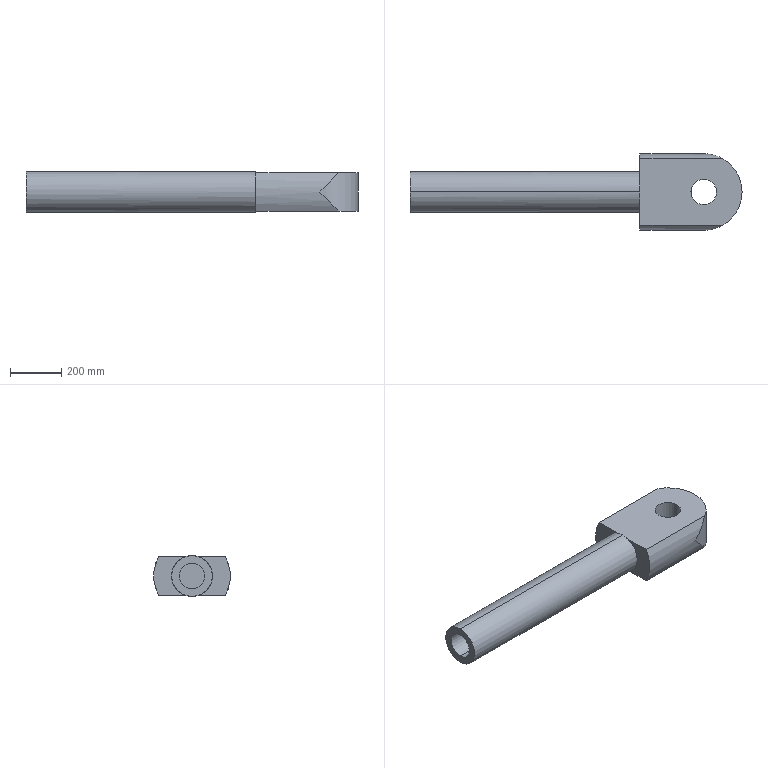Part | SolidWorks | features ICE 3, Extrusion 1 | 1 solid | 18 faces | box 1300 x 300 x 160 mm | volume 25837974 mm3 | cylinder 10 | plane 8 | commonest cylinder face diameters 100 x4 300 x4 160 x2
STEP:
#1=CARTESIAN_POINT('',(1200.,0.,-75.));
#2=VERTEX_POINT('',#1);
#3=CARTESIAN_POINT('',(1300.,0.,-75.));
#4=VERTEX_POINT('',#3);
#5=CARTESIAN_POINT('',(1250.,0.,-75.));
#6=DIRECTION('',(0.,0.,1.));
#7=DIRECTION('',(1.,0.,0.));
#8=AXIS2_PLACEMENT_3D('',#5,#6,#7);
#9=CIRCLE('',#8,50.);
#10=EDGE_CURVE('',#2,#4,#9,.T.);
#11=ORIENTED_EDGE('',*,*,#10,.F.);
#12=CARTESIAN_POINT('',(1200.,0.,75.));
#13=VERTEX_POINT('',#12);
#14=CARTESIAN_POINT('',(1200.,0.,-80.));
#15=DIRECTION('',(0.,0.,1.));
#16=VECTOR('',#15,1000.);
#17=LINE('',#14,#16);
#18=EDGE_CURVE('',#2,#13,#17,.T.);
#19=ORIENTED_EDGE('',*,*,#18,.T.);
#20=CARTESIAN_POINT('',(1300.,0.,75.));
#21=VERTEX_POINT('',#20);
#22=CARTESIAN_POINT('',(1250.,0.,75.));
#23=DIRECTION('',(0.,0.,-1.));
#24=DIRECTION('',(0.,1.,0.));
#25=AXIS2_PLACEMENT_3D('',#22,#23,#24);
#26=CIRCLE('',#25,50.);
#27=EDGE_CURVE('',#21,#13,#26,.T.);
#28=ORIENTED_EDGE('',*,*,#27,.F.);
#29=CARTESIAN_POINT('',(1300.,0.,-80.));
#30=DIRECTION('',(0.,0.,1.));
#31=VECTOR('',#30,1000.);
#32=LINE('',#29,#31);
#33=EDGE_CURVE('',#4,#21,#32,.T.);
#34=ORIENTED_EDGE('',*,*,#33,.F.);
#35=EDGE_LOOP('',(#11,#19,#28,#34));
#36=FACE_OUTER_BOUND('',#35,.T.);
#37=CARTESIAN_POINT('',(1250.,0.,-80.));
#38=DIRECTION('',(0.,0.,1.));
#39=DIRECTION('',(1.,0.,0.));
#40=AXIS2_PLACEMENT_3D('',#37,#38,#39);
#41=CYLINDRICAL_SURFACE('',#40,50.);
#42=ADVANCED_FACE('',(#36),#41,.F.);
#43=CARTESIAN_POINT('',(1325.,-129.904,-75.));
#44=VERTEX_POINT('',#43);
#45=CARTESIAN_POINT('',(1400.,0.,-75.));
#46=VERTEX_POINT('',#45);
#47=CARTESIAN_POINT('',(1250.,0.,-75.));
#48=DIRECTION('',(0.,0.,1.));
#49=DIRECTION('',(1.,0.,0.));
#50=AXIS2_PLACEMENT_3D('',#47,#48,#49);
#51=CIRCLE('',#50,150.);
#52=EDGE_CURVE('',#44,#46,#51,.T.);
#53=ORIENTED_EDGE('',*,*,#52,.T.);
#54=CARTESIAN_POINT('',(1400.,0.,75.));
#55=VERTEX_POINT('',#54);
#56=CARTESIAN_POINT('',(1400.,0.,-80.));
#57=DIRECTION('',(0.,0.,1.));
#58=VECTOR('',#57,1000.);
#59=LINE('',#56,#58);
#60=EDGE_CURVE('',#46,#55,#59,.T.);
#61=ORIENTED_EDGE('',*,*,#60,.T.);
#62=CARTESIAN_POINT('',(1325.,-129.904,75.));
#63=VERTEX_POINT('',#62);
#64=CARTESIAN_POINT('',(1250.,0.,75.));
#65=DIRECTION('',(0.,0.,-1.));
#66=DIRECTION('',(0.,1.,0.));
#67=AXIS2_PLACEMENT_3D('',#64,#65,#66);
#68=CIRCLE('',#67,150.);
#69=EDGE_CURVE('',#55,#63,#68,.T.);
#70=ORIENTED_EDGE('',*,*,#69,.T.);
#71=CARTESIAN_POINT('',(1250.,-150.,0.));
#72=VERTEX_POINT('',#71);
#73=CARTESIAN_POINT('',(1325.,-129.904,75.));
#74=CARTESIAN_POINT('',(1302.065,-143.146,52.065));
#75=CARTESIAN_POINT('',(1276.484,-150.,26.484));
#76=CARTESIAN_POINT('',(1250.,-150.,0.));
#77=(BOUNDED_CURVE()B_SPLINE_CURVE(3,(#73,#74,#75,#76),.UNSPECIFIED.,.F.,.F.)B_SPLINE_CURVE_WITH_KNOTS((4,4),(4.189,4.712),.UNSPECIFIED.)CURVE()GEOMETRIC_REPRESENTATION_ITEM()RATIONAL_B_SPLINE_CURVE((1.,0.9773,0.9773,1.))REPRESENTATION_ITEM(''));
#78=EDGE_CURVE('',#63,#72,#77,.T.);
#79=ORIENTED_EDGE('',*,*,#78,.T.);
#80=CARTESIAN_POINT('',(1250.,-150.,0.));
#81=CARTESIAN_POINT('',(1276.484,-150.,-26.484));
#82=CARTESIAN_POINT('',(1302.065,-143.146,-52.065));
#83=CARTESIAN_POINT('',(1325.,-129.904,-75.));
#84=(BOUNDED_CURVE()B_SPLINE_CURVE(3,(#80,#81,#82,#83),.UNSPECIFIED.,.F.,.T.)B_SPLINE_CURVE_WITH_KNOTS((4,4),(1.571,2.094),.UNSPECIFIED.)CURVE()GEOMETRIC_REPRESENTATION_ITEM()RATIONAL_B_SPLINE_CURVE((1.,0.9773,0.9773,1.))REPRESENTATION_ITEM(''));
#85=EDGE_CURVE('',#72,#44,#84,.T.);
#86=ORIENTED_EDGE('',*,*,#85,.T.);
#87=EDGE_LOOP('',(#53,#61,#70,#79,#86));
#88=FACE_OUTER_BOUND('',#87,.T.);
#89=CARTESIAN_POINT('',(1250.,0.,-80.));
#90=DIRECTION('',(0.,0.,1.));
#91=DIRECTION('',(1.,0.,0.));
#92=AXIS2_PLACEMENT_3D('',#89,#90,#91);
#93=CYLINDRICAL_SURFACE('',#92,150.);
#94=ADVANCED_FACE('',(#88),#93,.T.);
#95=CARTESIAN_POINT('',(1000.,0.,50.));
#96=VERTEX_POINT('',#95);
#97=CARTESIAN_POINT('',(1000.,0.,-50.));
#98=VERTEX_POINT('',#97);
#99=CARTESIAN_POINT('',(1000.,0.,0.));
#100=DIRECTION('',(1.,0.,0.));
#101=DIRECTION('',(0.,0.,-1.));
#102=AXIS2_PLACEMENT_3D('',#99,#100,#101);
#103=CIRCLE('',#102,50.);
#104=EDGE_CURVE('',#96,#98,#103,.T.);
#105=ORIENTED_EDGE('',*,*,#104,.T.);
#106=CARTESIAN_POINT('',(100.,0.,-50.));
#107=VERTEX_POINT('',#106);
#108=CARTESIAN_POINT('',(1000.,0.,-50.));
#109=DIRECTION('',(-1.,0.,0.));
#110=VECTOR('',#109,1000.);
#111=LINE('',#108,#110);
#112=EDGE_CURVE('',#98,#107,#111,.T.);
#113=ORIENTED_EDGE('',*,*,#112,.T.);
#114=CARTESIAN_POINT('',(100.,0.,50.));
#115=VERTEX_POINT('',#114);
#116=CARTESIAN_POINT('',(100.,0.,0.));
#117=DIRECTION('',(1.,0.,0.));
#118=DIRECTION('',(0.,0.,-1.));
#119=AXIS2_PLACEMENT_3D('',#116,#117,#118);
#120=CIRCLE('',#119,50.);
#121=EDGE_CURVE('',#115,#107,#120,.T.);
#122=ORIENTED_EDGE('',*,*,#121,.F.);
#123=CARTESIAN_POINT('',(1000.,0.,50.));
#124=DIRECTION('',(-1.,0.,0.));
#125=VECTOR('',#124,1000.);
#126=LINE('',#123,#125);
#127=EDGE_CURVE('',#96,#115,#126,.T.);
#128=ORIENTED_EDGE('',*,*,#127,.F.);
#129=EDGE_LOOP('',(#105,#113,#122,#128));
#130=FACE_OUTER_BOUND('',#129,.T.);
#131=CARTESIAN_POINT('',(1000.,0.,0.));
#132=DIRECTION('',(-1.,0.,0.));
#133=DIRECTION('',(0.,0.,1.));
#134=AXIS2_PLACEMENT_3D('',#131,#132,#133);
#135=CYLINDRICAL_SURFACE('',#134,50.);
#136=ADVANCED_FACE('',(#130),#135,.F.);
#137=CARTESIAN_POINT('',(1000.,0.,-80.));
#138=VERTEX_POINT('',#137);
#139=CARTESIAN_POINT('',(1000.,27.839,-75.));
#140=VERTEX_POINT('',#139);
#141=CARTESIAN_POINT('',(1000.,0.,0.));
#142=DIRECTION('',(1.,0.,0.));
#143=DIRECTION('',(0.,0.,-1.));
#144=AXIS2_PLACEMENT_3D('',#141,#142,#143);
#145=CIRCLE('',#144,80.);
#146=EDGE_CURVE('',#138,#140,#145,.T.);
#147=ORIENTED_EDGE('',*,*,#146,.F.);
#148=CARTESIAN_POINT('',(100.,0.,-80.));
#149=VERTEX_POINT('',#148);
#150=CARTESIAN_POINT('',(1000.,0.,-80.));
#151=DIRECTION('',(-1.,0.,0.));
#152=VECTOR('',#151,1000.);
#153=LINE('',#150,#152);
#154=EDGE_CURVE('',#138,#149,#153,.T.);
#155=ORIENTED_EDGE('',*,*,#154,.T.);
#156=CARTESIAN_POINT('',(100.,0.,80.));
#157=VERTEX_POINT('',#156);
#158=CARTESIAN_POINT('',(100.,0.,0.));
#159=DIRECTION('',(1.,0.,0.));
#160=DIRECTION('',(0.,0.,-1.));
#161=AXIS2_PLACEMENT_3D('',#158,#159,#160);
#162=CIRCLE('',#161,80.);
#163=EDGE_CURVE('',#149,#157,#162,.T.);
#164=ORIENTED_EDGE('',*,*,#163,.T.);
#165=CARTESIAN_POINT('',(1000.,0.,80.));
#166=VERTEX_POINT('',#165);
#167=CARTESIAN_POINT('',(1000.,0.,80.));
#168=DIRECTION('',(-1.,0.,0.));
#169=VECTOR('',#168,1000.);
#170=LINE('',#167,#169);
#171=EDGE_CURVE('',#166,#157,#170,.T.);
#172=ORIENTED_EDGE('',*,*,#171,.F.);
#173=CARTESIAN_POINT('',(1000.,27.839,75.));
#174=VERTEX_POINT('',#173);
#175=CARTESIAN_POINT('',(1000.,0.,0.));
#176=DIRECTION('',(1.,0.,0.));
#177=DIRECTION('',(0.,0.,-1.));
#178=AXIS2_PLACEMENT_3D('',#175,#176,#177);
#179=CIRCLE('',#178,80.);
#180=EDGE_CURVE('',#174,#166,#179,.T.);
#181=ORIENTED_EDGE('',*,*,#180,.F.);
#182=CARTESIAN_POINT('',(1000.,0.,0.));
#183=DIRECTION('',(1.,0.,0.));
#184=DIRECTION('',(0.,0.,-1.));
#185=AXIS2_PLACEMENT_3D('',#182,#183,#184);
#186=CIRCLE('',#185,80.);
#187=EDGE_CURVE('',#140,#174,#186,.T.);
#188=ORIENTED_EDGE('',*,*,#187,.F.);
#189=EDGE_LOOP('',(#147,#155,#164,#172,#181,#188));
#190=FACE_OUTER_BOUND('',#189,.T.);
#191=CARTESIAN_POINT('',(1000.,0.,0.));
#192=DIRECTION('',(-1.,0.,0.));
#193=DIRECTION('',(0.,0.,1.));
#194=AXIS2_PLACEMENT_3D('',#191,#192,#193);
#195=CYLINDRICAL_SURFACE('',#194,80.);
#196=ADVANCED_FACE('',(#190),#195,.T.);
#197=ORIENTED_EDGE('',*,*,#27,.T.);
#198=CARTESIAN_POINT('',(1250.,0.,75.));
#199=DIRECTION('',(0.,0.,-1.));
#200=DIRECTION('',(0.,1.,0.));
#201=AXIS2_PLACEMENT_3D('',#198,#199,#200);
#202=CIRCLE('',#201,50.);
#203=EDGE_CURVE('',#13,#21,#202,.T.);
#204=ORIENTED_EDGE('',*,*,#203,.T.);
#205=EDGE_LOOP('',(#197,#204));
#206=FACE_BOUND('',#205,.T.);
#207=CARTESIAN_POINT('',(1325.,129.904,75.));
#208=VERTEX_POINT('',#207);
#209=CARTESIAN_POINT('',(1250.,0.,75.));
#210=DIRECTION('',(0.,0.,-1.));
#211=DIRECTION('',(0.,1.,0.));
#212=AXIS2_PLACEMENT_3D('',#209,#210,#211);
#213=CIRCLE('',#212,150.);
#214=EDGE_CURVE('',#208,#55,#213,.T.);
#215=ORIENTED_EDGE('',*,*,#214,.F.);
#216=CARTESIAN_POINT('',(1000.,129.904,75.));
#217=VERTEX_POINT('',#216);
#218=CARTESIAN_POINT('',(1400.,129.904,75.));
#219=DIRECTION('',(-1.,0.,0.));
#220=VECTOR('',#219,1000.);
#221=LINE('',#218,#220);
#222=EDGE_CURVE('',#208,#217,#221,.T.);
#223=ORIENTED_EDGE('',*,*,#222,.T.);
#224=CARTESIAN_POINT('',(1000.,129.904,75.));
#225=DIRECTION('',(0.,-1.,0.));
#226=VECTOR('',#225,1000.);
#227=LINE('',#224,#226);
#228=EDGE_CURVE('',#217,#174,#227,.T.);
#229=ORIENTED_EDGE('',*,*,#228,.T.);
#230=CARTESIAN_POINT('',(1000.,-27.839,75.));
#231=VERTEX_POINT('',#230);
#232=CARTESIAN_POINT('',(1000.,129.904,75.));
#233=DIRECTION('',(0.,-1.,0.));
#234=VECTOR('',#233,1000.);
#235=LINE('',#232,#234);
#236=EDGE_CURVE('',#174,#231,#235,.T.);
#237=ORIENTED_EDGE('',*,*,#236,.T.);
#238=CARTESIAN_POINT('',(1000.,-129.904,75.));
#239=VERTEX_POINT('',#238);
#240=CARTESIAN_POINT('',(1000.,129.904,75.));
#241=DIRECTION('',(0.,-1.,0.));
#242=VECTOR('',#241,1000.);
#243=LINE('',#240,#242);
#244=EDGE_CURVE('',#231,#239,#243,.T.);
#245=ORIENTED_EDGE('',*,*,#244,.T.);
#246=CARTESIAN_POINT('',(1400.,-129.904,75.));
#247=DIRECTION('',(-1.,0.,0.));
#248=VECTOR('',#247,1000.);
#249=LINE('',#246,#248);
#250=EDGE_CURVE('',#63,#239,#249,.T.);
#251=ORIENTED_EDGE('',*,*,#250,.F.);
#252=ORIENTED_EDGE('',*,*,#69,.F.);
#253=EDGE_LOOP('',(#215,#223,#229,#237,#245,#251,#252));
#254=FACE_OUTER_BOUND('',#253,.T.);
#255=CARTESIAN_POINT('',(1400.,129.904,75.));
#256=DIRECTION('',(0.,0.,-1.));
#257=DIRECTION('',(0.,1.,0.));
#258=AXIS2_PLACEMENT_3D('',#255,#256,#257);
#259=PLANE('',#258);
#260=ADVANCED_FACE('',(#206,#254),#259,.F.);
#261=CARTESIAN_POINT('',(1250.,150.,0.));
#262=VERTEX_POINT('',#261);
#263=CARTESIAN_POINT('',(1250.,150.,0.));
#264=CARTESIAN_POINT('',(1276.484,150.,26.484));
#265=CARTESIAN_POINT('',(1302.065,143.146,52.065));
#266=CARTESIAN_POINT('',(1325.,129.904,75.));
#267=(BOUNDED_CURVE()B_SPLINE_CURVE(3,(#263,#264,#265,#266),.UNSPECIFIED.,.F.,.F.)B_SPLINE_CURVE_WITH_KNOTS((4,4),(1.571,2.094),.UNSPECIFIED.)CURVE()GEOMETRIC_REPRESENTATION_ITEM()RATIONAL_B_SPLINE_CURVE((1.,0.9773,0.9773,1.))REPRESENTATION_ITEM(''));
#268=EDGE_CURVE('',#262,#208,#267,.T.);
#269=ORIENTED_EDGE('',*,*,#268,.F.);
#270=CARTESIAN_POINT('',(1325.,129.904,-75.));
#271=VERTEX_POINT('',#270);
#272=CARTESIAN_POINT('',(1325.,129.904,-75.));
#273=CARTESIAN_POINT('',(1302.065,143.146,-52.065));
#274=CARTESIAN_POINT('',(1276.484,150.,-26.484));
#275=CARTESIAN_POINT('',(1250.,150.,0.));
#276=(BOUNDED_CURVE()B_SPLINE_CURVE(3,(#272,#273,#274,#275),.UNSPECIFIED.,.F.,.T.)B_SPLINE_CURVE_WITH_KNOTS((4,4),(4.189,4.712),.UNSPECIFIED.)CURVE()GEOMETRIC_REPRESENTATION_ITEM()RATIONAL_B_SPLINE_CURVE((1.,0.9773,0.9773,1.))REPRESENTATION_ITEM(''));
#277=EDGE_CURVE('',#271,#262,#276,.T.);
#278=ORIENTED_EDGE('',*,*,#277,.F.);
#279=CARTESIAN_POINT('',(1000.,129.904,-75.));
#280=VERTEX_POINT('',#279);
#281=CARTESIAN_POINT('',(1400.,129.904,-75.));
#282=DIRECTION('',(-1.,0.,0.));
#283=VECTOR('',#282,1000.);
#284=LINE('',#281,#283);
#285=EDGE_CURVE('',#271,#280,#284,.T.);
#286=ORIENTED_EDGE('',*,*,#285,.T.);
#287=CARTESIAN_POINT('',(1000.,0.,0.));
#288=DIRECTION('',(1.,0.,0.));
#289=DIRECTION('',(0.,0.,-1.));
#290=AXIS2_PLACEMENT_3D('',#287,#288,#289);
#291=CIRCLE('',#290,150.);
#292=EDGE_CURVE('',#280,#217,#291,.T.);
#293=ORIENTED_EDGE('',*,*,#292,.T.);
#294=ORIENTED_EDGE('',*,*,#222,.F.);
#295=EDGE_LOOP('',(#269,#278,#286,#293,#294));
#296=FACE_OUTER_BOUND('',#295,.T.);
#297=CARTESIAN_POINT('',(1400.,0.,0.));
#298=DIRECTION('',(-1.,0.,0.));
#299=DIRECTION('',(0.,0.,1.));
#300=AXIS2_PLACEMENT_3D('',#297,#298,#299);
#301=CYLINDRICAL_SURFACE('',#300,150.);
#302=ADVANCED_FACE('',(#296),#301,.T.);
#303=CARTESIAN_POINT('',(1250.,0.,-75.));
#304=DIRECTION('',(0.,0.,1.));
#305=DIRECTION('',(1.,0.,0.));
#306=AXIS2_PLACEMENT_3D('',#303,#304,#305);
#307=CIRCLE('',#306,50.);
#308=EDGE_CURVE('',#4,#2,#307,.T.);
#309=ORIENTED_EDGE('',*,*,#308,.T.);
#310=ORIENTED_EDGE('',*,*,#10,.T.);
#311=EDGE_LOOP('',(#309,#310));
#312=FACE_BOUND('',#311,.T.);
#313=ORIENTED_EDGE('',*,*,#52,.F.);
#314=CARTESIAN_POINT('',(1000.,-129.904,-75.));
#315=VERTEX_POINT('',#314);
#316=CARTESIAN_POINT('',(1400.,-129.904,-75.));
#317=DIRECTION('',(-1.,0.,0.));
#318=VECTOR('',#317,1000.);
#319=LINE('',#316,#318);
#320=EDGE_CURVE('',#44,#315,#319,.T.);
#321=ORIENTED_EDGE('',*,*,#320,.T.);
#322=CARTESIAN_POINT('',(1000.,-27.839,-75.));
#323=VERTEX_POINT('',#322);
#324=CARTESIAN_POINT('',(1000.,129.904,-75.));
#325=DIRECTION('',(0.,1.,0.));
#326=VECTOR('',#325,1000.);
#327=LINE('',#324,#326);
#328=EDGE_CURVE('',#315,#323,#327,.T.);
#329=ORIENTED_EDGE('',*,*,#328,.T.);
#330=CARTESIAN_POINT('',(1000.,129.904,-75.));
#331=DIRECTION('',(0.,1.,0.));
#332=VECTOR('',#331,1000.);
#333=LINE('',#330,#332);
#334=EDGE_CURVE('',#323,#140,#333,.T.);
#335=ORIENTED_EDGE('',*,*,#334,.T.);
#336=CARTESIAN_POINT('',(1000.,129.904,-75.));
#337=DIRECTION('',(0.,1.,0.));
#338=VECTOR('',#337,1000.);
#339=LINE('',#336,#338);
#340=EDGE_CURVE('',#140,#280,#339,.T.);
#341=ORIENTED_EDGE('',*,*,#340,.T.);
#342=ORIENTED_EDGE('',*,*,#285,.F.);
#343=CARTESIAN_POINT('',(1250.,0.,-75.));
#344=DIRECTION('',(0.,0.,1.));
#345=DIRECTION('',(1.,0.,0.));
#346=AXIS2_PLACEMENT_3D('',#343,#344,#345);
#347=CIRCLE('',#346,150.);
#348=EDGE_CURVE('',#46,#271,#347,.T.);
#349=ORIENTED_EDGE('',*,*,#348,.F.);
#350=EDGE_LOOP('',(#313,#321,#329,#335,#341,#342,#349));
#351=FACE_OUTER_BOUND('',#350,.T.);
#352=CARTESIAN_POINT('',(1400.,129.904,-75.));
#353=DIRECTION('',(0.,0.,1.));
#354=DIRECTION('',(1.,0.,0.));
#355=AXIS2_PLACEMENT_3D('',#352,#353,#354);
#356=PLANE('',#355);
#357=ADVANCED_FACE('',(#312,#351),#356,.F.);
#358=ORIENTED_EDGE('',*,*,#78,.F.);
#359=ORIENTED_EDGE('',*,*,#250,.T.);
#360=CARTESIAN_POINT('',(1000.,0.,0.));
#361=DIRECTION('',(1.,0.,0.));
#362=DIRECTION('',(0.,0.,-1.));
#363=AXIS2_PLACEMENT_3D('',#360,#361,#362);
#364=CIRCLE('',#363,150.);
#365=EDGE_CURVE('',#239,#315,#364,.T.);
#366=ORIENTED_EDGE('',*,*,#365,.T.);
#367=ORIENTED_EDGE('',*,*,#320,.F.);
#368=ORIENTED_EDGE('',*,*,#85,.F.);
#369=EDGE_LOOP('',(#358,#359,#366,#367,#368));
#370=FACE_OUTER_BOUND('',#369,.T.);
#371=CARTESIAN_POINT('',(1400.,0.,0.));
#372=DIRECTION('',(-1.,0.,0.));
#373=DIRECTION('',(0.,0.,1.));
#374=AXIS2_PLACEMENT_3D('',#371,#372,#373);
#375=CYLINDRICAL_SURFACE('',#374,150.);
#376=ADVANCED_FACE('',(#370),#375,.T.);
#377=ORIENTED_EDGE('',*,*,#236,.F.);
#378=ORIENTED_EDGE('',*,*,#180,.T.);
#379=CARTESIAN_POINT('',(1000.,0.,0.));
#380=DIRECTION('',(1.,0.,0.));
#381=DIRECTION('',(0.,0.,-1.));
#382=AXIS2_PLACEMENT_3D('',#379,#380,#381);
#383=CIRCLE('',#382,80.);
#384=EDGE_CURVE('',#166,#231,#383,.T.);
#385=ORIENTED_EDGE('',*,*,#384,.T.);
#386=EDGE_LOOP('',(#377,#378,#385));
#387=FACE_OUTER_BOUND('',#386,.T.);
#388=CARTESIAN_POINT('',(1000.,0.,0.));
#389=DIRECTION('',(1.,0.,0.));
#390=DIRECTION('',(0.,0.,-1.));
#391=AXIS2_PLACEMENT_3D('',#388,#389,#390);
#392=PLANE('',#391);
#393=ADVANCED_FACE('',(#387),#392,.T.);
#394=ORIENTED_EDGE('',*,*,#334,.F.);
#395=CARTESIAN_POINT('',(1000.,0.,0.));
#396=DIRECTION('',(1.,0.,0.));
#397=DIRECTION('',(0.,0.,-1.));
#398=AXIS2_PLACEMENT_3D('',#395,#396,#397);
#399=CIRCLE('',#398,80.);
#400=EDGE_CURVE('',#323,#138,#399,.T.);
#401=ORIENTED_EDGE('',*,*,#400,.T.);
#402=ORIENTED_EDGE('',*,*,#146,.T.);
#403=EDGE_LOOP('',(#394,#401,#402));
#404=FACE_OUTER_BOUND('',#403,.T.);
#405=CARTESIAN_POINT('',(1000.,0.,0.));
#406=DIRECTION('',(1.,0.,0.));
#407=DIRECTION('',(0.,0.,-1.));
#408=AXIS2_PLACEMENT_3D('',#405,#406,#407);
#409=PLANE('',#408);
#410=ADVANCED_FACE('',(#404),#409,.T.);
#411=CARTESIAN_POINT('',(100.,0.,0.));
#412=DIRECTION('',(1.,0.,0.));
#413=DIRECTION('',(0.,0.,-1.));
#414=AXIS2_PLACEMENT_3D('',#411,#412,#413);
#415=CIRCLE('',#414,80.);
#416=EDGE_CURVE('',#157,#149,#415,.T.);
#417=ORIENTED_EDGE('',*,*,#416,.F.);
#418=ORIENTED_EDGE('',*,*,#163,.F.);
#419=EDGE_LOOP('',(#417,#418));
#420=FACE_OUTER_BOUND('',#419,.T.);
#421=ORIENTED_EDGE('',*,*,#121,.T.);
#422=CARTESIAN_POINT('',(100.,0.,0.));
#423=DIRECTION('',(1.,0.,0.));
#424=DIRECTION('',(0.,0.,-1.));
#425=AXIS2_PLACEMENT_3D('',#422,#423,#424);
#426=CIRCLE('',#425,50.);
#427=EDGE_CURVE('',#107,#115,#426,.T.);
#428=ORIENTED_EDGE('',*,*,#427,.T.);
#429=EDGE_LOOP('',(#421,#428));
#430=FACE_BOUND('',#429,.T.);
#431=CARTESIAN_POINT('',(100.,0.,0.));
#432=DIRECTION('',(1.,0.,0.));
#433=DIRECTION('',(0.,0.,-1.));
#434=AXIS2_PLACEMENT_3D('',#431,#432,#433);
#435=PLANE('',#434);
#436=ADVANCED_FACE('',(#420,#430),#435,.F.);
#437=ORIENTED_EDGE('',*,*,#154,.F.);
#438=ORIENTED_EDGE('',*,*,#400,.F.);
#439=CARTESIAN_POINT('',(1000.,0.,0.));
#440=DIRECTION('',(1.,0.,0.));
#441=DIRECTION('',(0.,0.,-1.));
#442=AXIS2_PLACEMENT_3D('',#439,#440,#441);
#443=CIRCLE('',#442,80.);
#444=EDGE_CURVE('',#231,#323,#443,.T.);
#445=ORIENTED_EDGE('',*,*,#444,.F.);
#446=ORIENTED_EDGE('',*,*,#384,.F.);
#447=ORIENTED_EDGE('',*,*,#171,.T.);
#448=ORIENTED_EDGE('',*,*,#416,.T.);
#449=EDGE_LOOP('',(#437,#438,#445,#446,#447,#448));
#450=FACE_OUTER_BOUND('',#449,.T.);
#451=CARTESIAN_POINT('',(1000.,0.,0.));
#452=DIRECTION('',(-1.,0.,0.));
#453=DIRECTION('',(0.,0.,1.));
#454=AXIS2_PLACEMENT_3D('',#451,#452,#453);
#455=CYLINDRICAL_SURFACE('',#454,80.);
#456=ADVANCED_FACE('',(#450),#455,.T.);
#457=ORIENTED_EDGE('',*,*,#112,.F.);
#458=CARTESIAN_POINT('',(1000.,0.,0.));
#459=DIRECTION('',(1.,0.,0.));
#460=DIRECTION('',(0.,0.,-1.));
#461=AXIS2_PLACEMENT_3D('',#458,#459,#460);
#462=CIRCLE('',#461,50.);
#463=EDGE_CURVE('',#98,#96,#462,.T.);
#464=ORIENTED_EDGE('',*,*,#463,.T.);
#465=ORIENTED_EDGE('',*,*,#127,.T.);
#466=ORIENTED_EDGE('',*,*,#427,.F.);
#467=EDGE_LOOP('',(#457,#464,#465,#466));
#468=FACE_OUTER_BOUND('',#467,.T.);
#469=CARTESIAN_POINT('',(1000.,0.,0.));
#470=DIRECTION('',(-1.,0.,0.));
#471=DIRECTION('',(0.,0.,1.));
#472=AXIS2_PLACEMENT_3D('',#469,#470,#471);
#473=CYLINDRICAL_SURFACE('',#472,50.);
#474=ADVANCED_FACE('',(#468),#473,.F.);
#475=ORIENTED_EDGE('',*,*,#244,.F.);
#476=ORIENTED_EDGE('',*,*,#444,.T.);
#477=ORIENTED_EDGE('',*,*,#328,.F.);
#478=ORIENTED_EDGE('',*,*,#365,.F.);
#479=EDGE_LOOP('',(#475,#476,#477,#478));
#480=FACE_OUTER_BOUND('',#479,.T.);
#481=CARTESIAN_POINT('',(1000.,0.,0.));
#482=DIRECTION('',(1.,0.,0.));
#483=DIRECTION('',(0.,0.,-1.));
#484=AXIS2_PLACEMENT_3D('',#481,#482,#483);
#485=PLANE('',#484);
#486=ADVANCED_FACE('',(#480),#485,.F.);
#487=ORIENTED_EDGE('',*,*,#340,.F.);
#488=ORIENTED_EDGE('',*,*,#187,.T.);
#489=ORIENTED_EDGE('',*,*,#228,.F.);
#490=ORIENTED_EDGE('',*,*,#292,.F.);
#491=EDGE_LOOP('',(#487,#488,#489,#490));
#492=FACE_OUTER_BOUND('',#491,.T.);
#493=CARTESIAN_POINT('',(1000.,0.,0.));
#494=DIRECTION('',(1.,0.,0.));
#495=DIRECTION('',(0.,0.,-1.));
#496=AXIS2_PLACEMENT_3D('',#493,#494,#495);
#497=PLANE('',#496);
#498=ADVANCED_FACE('',(#492),#497,.F.);
#499=ORIENTED_EDGE('',*,*,#104,.F.);
#500=ORIENTED_EDGE('',*,*,#463,.F.);
#501=EDGE_LOOP('',(#499,#500));
#502=FACE_OUTER_BOUND('',#501,.T.);
#503=CARTESIAN_POINT('',(1000.,0.,0.));
#504=DIRECTION('',(1.,0.,0.));
#505=DIRECTION('',(0.,0.,-1.));
#506=AXIS2_PLACEMENT_3D('',#503,#504,#505);
#507=PLANE('',#506);
#508=ADVANCED_FACE('',(#502),#507,.F.);
#509=ORIENTED_EDGE('',*,*,#60,.F.);
#510=ORIENTED_EDGE('',*,*,#348,.T.);
#511=ORIENTED_EDGE('',*,*,#277,.T.);
#512=ORIENTED_EDGE('',*,*,#268,.T.);
#513=ORIENTED_EDGE('',*,*,#214,.T.);
#514=EDGE_LOOP('',(#509,#510,#511,#512,#513));
#515=FACE_OUTER_BOUND('',#514,.T.);
#516=CARTESIAN_POINT('',(1250.,0.,-80.));
#517=DIRECTION('',(0.,0.,1.));
#518=DIRECTION('',(1.,0.,0.));
#519=AXIS2_PLACEMENT_3D('',#516,#517,#518);
#520=CYLINDRICAL_SURFACE('',#519,150.);
#521=ADVANCED_FACE('',(#515),#520,.T.);
#522=ORIENTED_EDGE('',*,*,#18,.F.);
#523=ORIENTED_EDGE('',*,*,#308,.F.);
#524=ORIENTED_EDGE('',*,*,#33,.T.);
#525=ORIENTED_EDGE('',*,*,#203,.F.);
#526=EDGE_LOOP('',(#522,#523,#524,#525));
#527=FACE_OUTER_BOUND('',#526,.T.);
#528=CARTESIAN_POINT('',(1250.,0.,-80.));
#529=DIRECTION('',(0.,0.,1.));
#530=DIRECTION('',(1.,0.,0.));
#531=AXIS2_PLACEMENT_3D('',#528,#529,#530);
#532=CYLINDRICAL_SURFACE('',#531,50.);
#533=ADVANCED_FACE('',(#527),#532,.F.);
#534=CLOSED_SHELL('',(#42,#94,#136,#196,#260,#302,#357,#376,#393,#410,#436,#456,#474,#486,#498,#508,#521,#533));
#535=MANIFOLD_SOLID_BREP('',#534);
#536=CARTESIAN_POINT('',(0.,0.,0.));
#537=DIRECTION('',(0.,0.,1.));
#538=DIRECTION('',(1.,0.,0.));
#539=AXIS2_PLACEMENT_3D('',#536,#537,#538);
#540=(LENGTH_UNIT()NAMED_UNIT(*)SI_UNIT(.MILLI.,.METRE.));
#541=UNCERTAINTY_MEASURE_WITH_UNIT(LENGTH_MEASURE(0.00001),#540,'','');
#542=(NAMED_UNIT(*)PLANE_ANGLE_UNIT()SI_UNIT($,.RADIAN.));
#543=(NAMED_UNIT(*)SI_UNIT($,.STERADIAN.)SOLID_ANGLE_UNIT());
#544=(GEOMETRIC_REPRESENTATION_CONTEXT(3)GLOBAL_UNCERTAINTY_ASSIGNED_CONTEXT((#541))GLOBAL_UNIT_ASSIGNED_CONTEXT((#540,#542,#543))REPRESENTATION_CONTEXT('',''));
#545=ADVANCED_BREP_SHAPE_REPRESENTATION('',(#535,#539),#544);